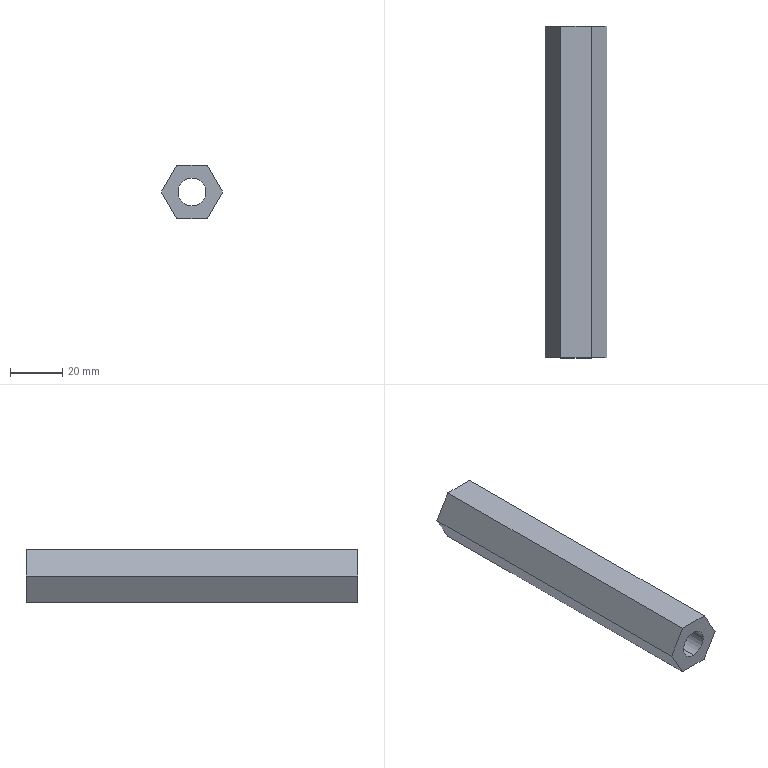Part | SolidWorks | features Extrusion 1, ICE 1, Scale 1 | 1 solid | 10 faces | box 23.464 x 127 x 20.32 mm | volume 34061 mm3 | plane 8 | cylinder 2 | commonest cylinder face diameters 10.668 x2
STEP:
#1=CARTESIAN_POINT('',(0.,127.,5.334));
#2=VERTEX_POINT('',#1);
#3=CARTESIAN_POINT('',(0.,127.,-5.334));
#4=VERTEX_POINT('',#3);
#5=CARTESIAN_POINT('',(0.,127.,0.));
#6=DIRECTION('',(0.,-1.,0.));
#7=DIRECTION('',(0.,0.,1.));
#8=AXIS2_PLACEMENT_3D('',#5,#6,#7);
#9=CIRCLE('',#8,5.334);
#10=EDGE_CURVE('',#2,#4,#9,.T.);
#11=ORIENTED_EDGE('',*,*,#10,.F.);
#12=CARTESIAN_POINT('',(0.,0.,5.334));
#13=VERTEX_POINT('',#12);
#14=CARTESIAN_POINT('',(0.,254.,5.334));
#15=DIRECTION('',(0.,-1.,0.));
#16=VECTOR('',#15,1000.);
#17=LINE('',#14,#16);
#18=EDGE_CURVE('',#2,#13,#17,.T.);
#19=ORIENTED_EDGE('',*,*,#18,.T.);
#20=CARTESIAN_POINT('',(0.,0.,-5.334));
#21=VERTEX_POINT('',#20);
#22=CARTESIAN_POINT('',(0.,0.,0.));
#23=DIRECTION('',(0.,1.,0.));
#24=DIRECTION('',(0.,0.,1.));
#25=AXIS2_PLACEMENT_3D('',#22,#23,#24);
#26=CIRCLE('',#25,5.334);
#27=EDGE_CURVE('',#21,#13,#26,.T.);
#28=ORIENTED_EDGE('',*,*,#27,.F.);
#29=CARTESIAN_POINT('',(0.,254.,-5.334));
#30=DIRECTION('',(0.,-1.,0.));
#31=VECTOR('',#30,1000.);
#32=LINE('',#29,#31);
#33=EDGE_CURVE('',#4,#21,#32,.T.);
#34=ORIENTED_EDGE('',*,*,#33,.F.);
#35=EDGE_LOOP('',(#11,#19,#28,#34));
#36=FACE_OUTER_BOUND('',#35,.T.);
#37=CARTESIAN_POINT('',(0.,254.,0.));
#38=DIRECTION('',(0.,-1.,0.));
#39=DIRECTION('',(0.,0.,-1.));
#40=AXIS2_PLACEMENT_3D('',#37,#38,#39);
#41=CYLINDRICAL_SURFACE('',#40,5.334);
#42=ADVANCED_FACE('',(#36),#41,.F.);
#43=CARTESIAN_POINT('',(-5.866,127.,10.16));
#44=VERTEX_POINT('',#43);
#45=CARTESIAN_POINT('',(5.866,127.,10.16));
#46=VERTEX_POINT('',#45);
#47=CARTESIAN_POINT('',(-5.866,127.,10.16));
#48=DIRECTION('',(1.,0.,0.));
#49=VECTOR('',#48,1000.);
#50=LINE('',#47,#49);
#51=EDGE_CURVE('',#44,#46,#50,.T.);
#52=ORIENTED_EDGE('',*,*,#51,.T.);
#53=CARTESIAN_POINT('',(11.732,127.,0.));
#54=VERTEX_POINT('',#53);
#55=CARTESIAN_POINT('',(5.866,127.,10.16));
#56=DIRECTION('',(0.5,0.,-0.866));
#57=VECTOR('',#56,1000.);
#58=LINE('',#55,#57);
#59=EDGE_CURVE('',#46,#54,#58,.T.);
#60=ORIENTED_EDGE('',*,*,#59,.T.);
#61=CARTESIAN_POINT('',(5.866,127.,-10.16));
#62=VERTEX_POINT('',#61);
#63=CARTESIAN_POINT('',(11.732,127.,0.));
#64=DIRECTION('',(-0.5,0.,-0.866));
#65=VECTOR('',#64,1000.);
#66=LINE('',#63,#65);
#67=EDGE_CURVE('',#54,#62,#66,.T.);
#68=ORIENTED_EDGE('',*,*,#67,.T.);
#69=CARTESIAN_POINT('',(-5.866,127.,-10.16));
#70=VERTEX_POINT('',#69);
#71=CARTESIAN_POINT('',(5.866,127.,-10.16));
#72=DIRECTION('',(-1.,0.,0.));
#73=VECTOR('',#72,1000.);
#74=LINE('',#71,#73);
#75=EDGE_CURVE('',#62,#70,#74,.T.);
#76=ORIENTED_EDGE('',*,*,#75,.T.);
#77=CARTESIAN_POINT('',(-11.732,127.,0.));
#78=VERTEX_POINT('',#77);
#79=CARTESIAN_POINT('',(-5.866,127.,-10.16));
#80=DIRECTION('',(-0.5,0.,0.866));
#81=VECTOR('',#80,1000.);
#82=LINE('',#79,#81);
#83=EDGE_CURVE('',#70,#78,#82,.T.);
#84=ORIENTED_EDGE('',*,*,#83,.T.);
#85=CARTESIAN_POINT('',(-11.732,127.,0.));
#86=DIRECTION('',(0.5,0.,0.866));
#87=VECTOR('',#86,1000.);
#88=LINE('',#85,#87);
#89=EDGE_CURVE('',#78,#44,#88,.T.);
#90=ORIENTED_EDGE('',*,*,#89,.T.);
#91=EDGE_LOOP('',(#52,#60,#68,#76,#84,#90));
#92=FACE_OUTER_BOUND('',#91,.T.);
#93=CARTESIAN_POINT('',(0.,127.,0.));
#94=DIRECTION('',(0.,-1.,0.));
#95=DIRECTION('',(0.,0.,1.));
#96=AXIS2_PLACEMENT_3D('',#93,#94,#95);
#97=CIRCLE('',#96,5.334);
#98=EDGE_CURVE('',#4,#2,#97,.T.);
#99=ORIENTED_EDGE('',*,*,#98,.T.);
#100=ORIENTED_EDGE('',*,*,#10,.T.);
#101=EDGE_LOOP('',(#99,#100));
#102=FACE_BOUND('',#101,.T.);
#103=CARTESIAN_POINT('',(0.,127.,0.));
#104=DIRECTION('',(0.,1.,0.));
#105=DIRECTION('',(0.,0.,1.));
#106=AXIS2_PLACEMENT_3D('',#103,#104,#105);
#107=PLANE('',#106);
#108=ADVANCED_FACE('',(#92,#102),#107,.T.);
#109=CARTESIAN_POINT('',(-5.866,0.,10.16));
#110=VERTEX_POINT('',#109);
#111=CARTESIAN_POINT('',(5.866,0.,10.16));
#112=VERTEX_POINT('',#111);
#113=CARTESIAN_POINT('',(-5.866,0.,10.16));
#114=DIRECTION('',(1.,0.,0.));
#115=VECTOR('',#114,1000.);
#116=LINE('',#113,#115);
#117=EDGE_CURVE('',#110,#112,#116,.T.);
#118=ORIENTED_EDGE('',*,*,#117,.F.);
#119=CARTESIAN_POINT('',(-11.732,0.,0.));
#120=VERTEX_POINT('',#119);
#121=CARTESIAN_POINT('',(-11.732,0.,0.));
#122=DIRECTION('',(0.5,0.,0.866));
#123=VECTOR('',#122,1000.);
#124=LINE('',#121,#123);
#125=EDGE_CURVE('',#120,#110,#124,.T.);
#126=ORIENTED_EDGE('',*,*,#125,.F.);
#127=CARTESIAN_POINT('',(-5.866,0.,-10.16));
#128=VERTEX_POINT('',#127);
#129=CARTESIAN_POINT('',(-5.866,0.,-10.16));
#130=DIRECTION('',(-0.5,0.,0.866));
#131=VECTOR('',#130,1000.);
#132=LINE('',#129,#131);
#133=EDGE_CURVE('',#128,#120,#132,.T.);
#134=ORIENTED_EDGE('',*,*,#133,.F.);
#135=CARTESIAN_POINT('',(5.866,0.,-10.16));
#136=VERTEX_POINT('',#135);
#137=CARTESIAN_POINT('',(5.866,0.,-10.16));
#138=DIRECTION('',(-1.,0.,0.));
#139=VECTOR('',#138,1000.);
#140=LINE('',#137,#139);
#141=EDGE_CURVE('',#136,#128,#140,.T.);
#142=ORIENTED_EDGE('',*,*,#141,.F.);
#143=CARTESIAN_POINT('',(11.732,0.,0.));
#144=VERTEX_POINT('',#143);
#145=CARTESIAN_POINT('',(11.732,0.,0.));
#146=DIRECTION('',(-0.5,0.,-0.866));
#147=VECTOR('',#146,1000.);
#148=LINE('',#145,#147);
#149=EDGE_CURVE('',#144,#136,#148,.T.);
#150=ORIENTED_EDGE('',*,*,#149,.F.);
#151=CARTESIAN_POINT('',(5.866,0.,10.16));
#152=DIRECTION('',(0.5,0.,-0.866));
#153=VECTOR('',#152,1000.);
#154=LINE('',#151,#153);
#155=EDGE_CURVE('',#112,#144,#154,.T.);
#156=ORIENTED_EDGE('',*,*,#155,.F.);
#157=EDGE_LOOP('',(#118,#126,#134,#142,#150,#156));
#158=FACE_OUTER_BOUND('',#157,.T.);
#159=ORIENTED_EDGE('',*,*,#27,.T.);
#160=CARTESIAN_POINT('',(0.,0.,0.));
#161=DIRECTION('',(0.,1.,0.));
#162=DIRECTION('',(0.,0.,1.));
#163=AXIS2_PLACEMENT_3D('',#160,#161,#162);
#164=CIRCLE('',#163,5.334);
#165=EDGE_CURVE('',#13,#21,#164,.T.);
#166=ORIENTED_EDGE('',*,*,#165,.T.);
#167=EDGE_LOOP('',(#159,#166));
#168=FACE_BOUND('',#167,.T.);
#169=CARTESIAN_POINT('',(0.,0.,0.));
#170=DIRECTION('',(0.,1.,0.));
#171=DIRECTION('',(0.,0.,1.));
#172=AXIS2_PLACEMENT_3D('',#169,#170,#171);
#173=PLANE('',#172);
#174=ADVANCED_FACE('',(#158,#168),#173,.F.);
#175=ORIENTED_EDGE('',*,*,#117,.T.);
#176=CARTESIAN_POINT('',(5.866,127.,10.16));
#177=DIRECTION('',(0.,-1.,0.));
#178=VECTOR('',#177,1000.);
#179=LINE('',#176,#178);
#180=EDGE_CURVE('',#46,#112,#179,.T.);
#181=ORIENTED_EDGE('',*,*,#180,.F.);
#182=ORIENTED_EDGE('',*,*,#51,.F.);
#183=CARTESIAN_POINT('',(-5.866,127.,10.16));
#184=DIRECTION('',(0.,-1.,0.));
#185=VECTOR('',#184,1000.);
#186=LINE('',#183,#185);
#187=EDGE_CURVE('',#44,#110,#186,.T.);
#188=ORIENTED_EDGE('',*,*,#187,.T.);
#189=EDGE_LOOP('',(#175,#181,#182,#188));
#190=FACE_OUTER_BOUND('',#189,.T.);
#191=CARTESIAN_POINT('',(-5.866,127.,10.16));
#192=DIRECTION('',(0.,0.,-1.));
#193=DIRECTION('',(-1.,0.,0.));
#194=AXIS2_PLACEMENT_3D('',#191,#192,#193);
#195=PLANE('',#194);
#196=ADVANCED_FACE('',(#190),#195,.F.);
#197=ORIENTED_EDGE('',*,*,#155,.T.);
#198=CARTESIAN_POINT('',(11.732,127.,0.));
#199=DIRECTION('',(0.,-1.,0.));
#200=VECTOR('',#199,1000.);
#201=LINE('',#198,#200);
#202=EDGE_CURVE('',#54,#144,#201,.T.);
#203=ORIENTED_EDGE('',*,*,#202,.F.);
#204=ORIENTED_EDGE('',*,*,#59,.F.);
#205=ORIENTED_EDGE('',*,*,#180,.T.);
#206=EDGE_LOOP('',(#197,#203,#204,#205));
#207=FACE_OUTER_BOUND('',#206,.T.);
#208=CARTESIAN_POINT('',(5.866,127.,10.16));
#209=DIRECTION('',(-0.866,0.,-0.5));
#210=DIRECTION('',(-0.5,0.,0.866));
#211=AXIS2_PLACEMENT_3D('',#208,#209,#210);
#212=PLANE('',#211);
#213=ADVANCED_FACE('',(#207),#212,.F.);
#214=ORIENTED_EDGE('',*,*,#149,.T.);
#215=CARTESIAN_POINT('',(5.866,127.,-10.16));
#216=DIRECTION('',(0.,-1.,0.));
#217=VECTOR('',#216,1000.);
#218=LINE('',#215,#217);
#219=EDGE_CURVE('',#62,#136,#218,.T.);
#220=ORIENTED_EDGE('',*,*,#219,.F.);
#221=ORIENTED_EDGE('',*,*,#67,.F.);
#222=ORIENTED_EDGE('',*,*,#202,.T.);
#223=EDGE_LOOP('',(#214,#220,#221,#222));
#224=FACE_OUTER_BOUND('',#223,.T.);
#225=CARTESIAN_POINT('',(11.732,127.,0.));
#226=DIRECTION('',(-0.866,0.,0.5));
#227=DIRECTION('',(0.5,0.,0.866));
#228=AXIS2_PLACEMENT_3D('',#225,#226,#227);
#229=PLANE('',#228);
#230=ADVANCED_FACE('',(#224),#229,.F.);
#231=ORIENTED_EDGE('',*,*,#141,.T.);
#232=CARTESIAN_POINT('',(-5.866,127.,-10.16));
#233=DIRECTION('',(0.,-1.,0.));
#234=VECTOR('',#233,1000.);
#235=LINE('',#232,#234);
#236=EDGE_CURVE('',#70,#128,#235,.T.);
#237=ORIENTED_EDGE('',*,*,#236,.F.);
#238=ORIENTED_EDGE('',*,*,#75,.F.);
#239=ORIENTED_EDGE('',*,*,#219,.T.);
#240=EDGE_LOOP('',(#231,#237,#238,#239));
#241=FACE_OUTER_BOUND('',#240,.T.);
#242=CARTESIAN_POINT('',(5.866,127.,-10.16));
#243=DIRECTION('',(0.,0.,1.));
#244=DIRECTION('',(1.,0.,0.));
#245=AXIS2_PLACEMENT_3D('',#242,#243,#244);
#246=PLANE('',#245);
#247=ADVANCED_FACE('',(#241),#246,.F.);
#248=ORIENTED_EDGE('',*,*,#133,.T.);
#249=CARTESIAN_POINT('',(-11.732,127.,0.));
#250=DIRECTION('',(0.,-1.,0.));
#251=VECTOR('',#250,1000.);
#252=LINE('',#249,#251);
#253=EDGE_CURVE('',#78,#120,#252,.T.);
#254=ORIENTED_EDGE('',*,*,#253,.F.);
#255=ORIENTED_EDGE('',*,*,#83,.F.);
#256=ORIENTED_EDGE('',*,*,#236,.T.);
#257=EDGE_LOOP('',(#248,#254,#255,#256));
#258=FACE_OUTER_BOUND('',#257,.T.);
#259=CARTESIAN_POINT('',(-5.866,127.,-10.16));
#260=DIRECTION('',(0.866,0.,0.5));
#261=DIRECTION('',(0.5,0.,-0.866));
#262=AXIS2_PLACEMENT_3D('',#259,#260,#261);
#263=PLANE('',#262);
#264=ADVANCED_FACE('',(#258),#263,.F.);
#265=ORIENTED_EDGE('',*,*,#125,.T.);
#266=ORIENTED_EDGE('',*,*,#187,.F.);
#267=ORIENTED_EDGE('',*,*,#89,.F.);
#268=ORIENTED_EDGE('',*,*,#253,.T.);
#269=EDGE_LOOP('',(#265,#266,#267,#268));
#270=FACE_OUTER_BOUND('',#269,.T.);
#271=CARTESIAN_POINT('',(-11.732,127.,0.));
#272=DIRECTION('',(0.866,0.,-0.5));
#273=DIRECTION('',(-0.5,0.,-0.866));
#274=AXIS2_PLACEMENT_3D('',#271,#272,#273);
#275=PLANE('',#274);
#276=ADVANCED_FACE('',(#270),#275,.F.);
#277=ORIENTED_EDGE('',*,*,#18,.F.);
#278=ORIENTED_EDGE('',*,*,#98,.F.);
#279=ORIENTED_EDGE('',*,*,#33,.T.);
#280=ORIENTED_EDGE('',*,*,#165,.F.);
#281=EDGE_LOOP('',(#277,#278,#279,#280));
#282=FACE_OUTER_BOUND('',#281,.T.);
#283=CARTESIAN_POINT('',(0.,254.,0.));
#284=DIRECTION('',(0.,-1.,0.));
#285=DIRECTION('',(0.,0.,-1.));
#286=AXIS2_PLACEMENT_3D('',#283,#284,#285);
#287=CYLINDRICAL_SURFACE('',#286,5.334);
#288=ADVANCED_FACE('',(#282),#287,.F.);
#289=CLOSED_SHELL('',(#42,#108,#174,#196,#213,#230,#247,#264,#276,#288));
#290=MANIFOLD_SOLID_BREP('',#289);
#291=CARTESIAN_POINT('',(0.,0.,0.));
#292=DIRECTION('',(0.,0.,1.));
#293=DIRECTION('',(1.,0.,0.));
#294=AXIS2_PLACEMENT_3D('',#291,#292,#293);
#295=(LENGTH_UNIT()NAMED_UNIT(*)SI_UNIT(.MILLI.,.METRE.));
#296=UNCERTAINTY_MEASURE_WITH_UNIT(LENGTH_MEASURE(0.00001),#295,'','');
#297=(NAMED_UNIT(*)PLANE_ANGLE_UNIT()SI_UNIT($,.RADIAN.));
#298=(NAMED_UNIT(*)SI_UNIT($,.STERADIAN.)SOLID_ANGLE_UNIT());
#299=(GEOMETRIC_REPRESENTATION_CONTEXT(3)GLOBAL_UNCERTAINTY_ASSIGNED_CONTEXT((#296))GLOBAL_UNIT_ASSIGNED_CONTEXT((#295,#297,#298))REPRESENTATION_CONTEXT('',''));
#300=ADVANCED_BREP_SHAPE_REPRESENTATION('',(#290,#294),#299);